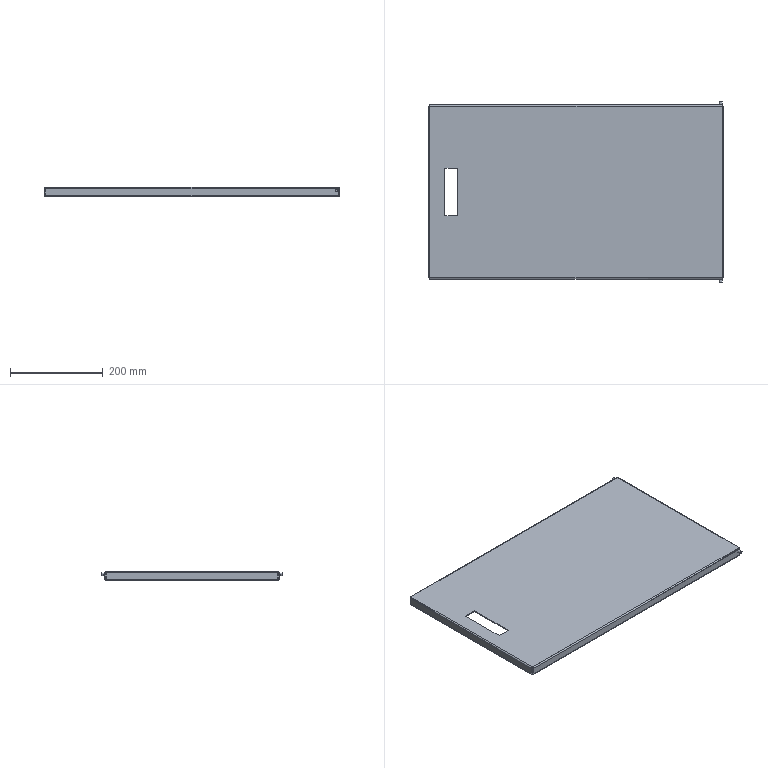Part | SolidWorks | features EdgeFlange 2, MoveCopyBody 2, Stock 2, FlatPattern 1, ICE 1, SMBaseFlange 1, SheetMetal 1 | 3 solids | 102 faces | box 636 x 390 x 20 mm | volume 609250 mm3 | plane 50 | cylinder 28 | spline 16 | cone 8 | commonest cylinder face diameters 1.473 x8 5.473 x8 6 x8 8 x4